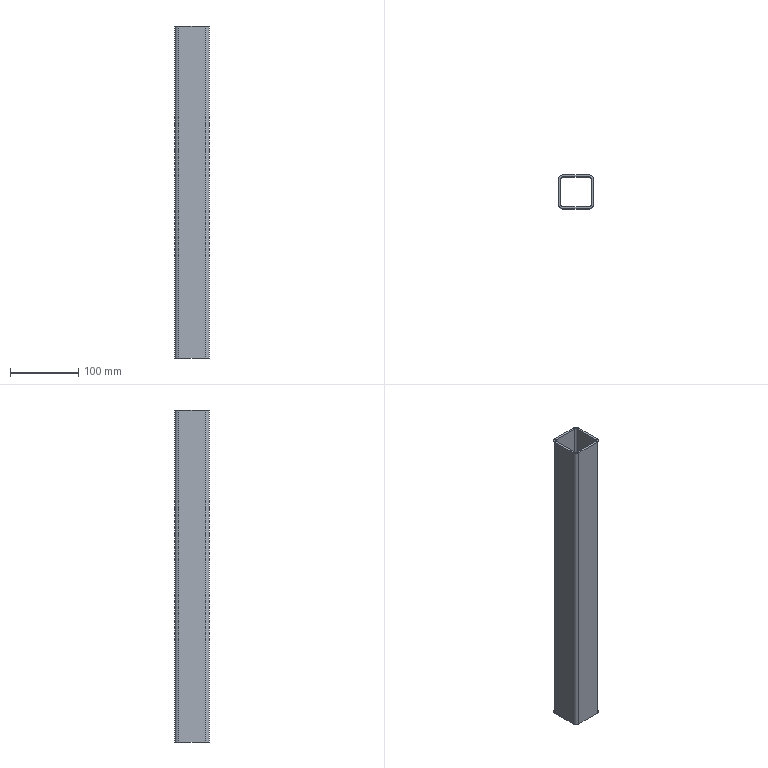Part | SolidWorks | 1 solid | 18 faces | box 50 x 50 x 485 mm | volume 262299 mm3 | plane 10 | cylinder 8 | commonest cylinder face diameters 6 x4 12 x4
STEP:
#1=CARTESIAN_POINT('',(19.,25.,242.5));
#2=VERTEX_POINT('',#1);
#3=CARTESIAN_POINT('',(25.,19.,242.5));
#4=VERTEX_POINT('',#3);
#5=CARTESIAN_POINT('',(19.,19.,242.5));
#6=DIRECTION('',(0.,0.,-1.));
#7=DIRECTION('',(-1.,0.,0.));
#8=AXIS2_PLACEMENT_3D('',#5,#6,#7);
#9=CIRCLE('',#8,6.);
#10=EDGE_CURVE('',#2,#4,#9,.T.);
#11=ORIENTED_EDGE('',*,*,#10,.T.);
#12=CARTESIAN_POINT('',(25.,19.,-242.5));
#13=VERTEX_POINT('',#12);
#14=CARTESIAN_POINT('',(25.,19.,-242.5));
#15=DIRECTION('',(0.,0.,1.));
#16=VECTOR('',#15,1000.);
#17=LINE('',#14,#16);
#18=EDGE_CURVE('',#13,#4,#17,.T.);
#19=ORIENTED_EDGE('',*,*,#18,.F.);
#20=CARTESIAN_POINT('',(19.,25.,-242.5));
#21=VERTEX_POINT('',#20);
#22=CARTESIAN_POINT('',(19.,19.,-242.5));
#23=DIRECTION('',(0.,0.,-1.));
#24=DIRECTION('',(-1.,0.,0.));
#25=AXIS2_PLACEMENT_3D('',#22,#23,#24);
#26=CIRCLE('',#25,6.);
#27=EDGE_CURVE('',#21,#13,#26,.T.);
#28=ORIENTED_EDGE('',*,*,#27,.F.);
#29=CARTESIAN_POINT('',(19.,25.,-242.5));
#30=DIRECTION('',(0.,0.,1.));
#31=VECTOR('',#30,1000.);
#32=LINE('',#29,#31);
#33=EDGE_CURVE('',#21,#2,#32,.T.);
#34=ORIENTED_EDGE('',*,*,#33,.T.);
#35=EDGE_LOOP('',(#11,#19,#28,#34));
#36=FACE_OUTER_BOUND('',#35,.T.);
#37=CARTESIAN_POINT('',(19.,19.,-242.5));
#38=DIRECTION('',(0.,0.,1.));
#39=DIRECTION('',(1.,0.,0.));
#40=AXIS2_PLACEMENT_3D('',#37,#38,#39);
#41=CYLINDRICAL_SURFACE('',#40,6.);
#42=ADVANCED_FACE('',(#36),#41,.T.);
#43=CARTESIAN_POINT('',(25.,-19.,242.5));
#44=VERTEX_POINT('',#43);
#45=CARTESIAN_POINT('',(25.,19.,242.5));
#46=DIRECTION('',(0.,-1.,0.));
#47=VECTOR('',#46,1000.);
#48=LINE('',#45,#47);
#49=EDGE_CURVE('',#4,#44,#48,.T.);
#50=ORIENTED_EDGE('',*,*,#49,.T.);
#51=CARTESIAN_POINT('',(25.,-19.,-242.5));
#52=VERTEX_POINT('',#51);
#53=CARTESIAN_POINT('',(25.,-19.,-242.5));
#54=DIRECTION('',(0.,0.,1.));
#55=VECTOR('',#54,1000.);
#56=LINE('',#53,#55);
#57=EDGE_CURVE('',#52,#44,#56,.T.);
#58=ORIENTED_EDGE('',*,*,#57,.F.);
#59=CARTESIAN_POINT('',(25.,19.,-242.5));
#60=DIRECTION('',(0.,-1.,0.));
#61=VECTOR('',#60,1000.);
#62=LINE('',#59,#61);
#63=EDGE_CURVE('',#13,#52,#62,.T.);
#64=ORIENTED_EDGE('',*,*,#63,.F.);
#65=ORIENTED_EDGE('',*,*,#18,.T.);
#66=EDGE_LOOP('',(#50,#58,#64,#65));
#67=FACE_OUTER_BOUND('',#66,.T.);
#68=CARTESIAN_POINT('',(25.,19.,-242.5));
#69=DIRECTION('',(-1.,0.,0.));
#70=DIRECTION('',(0.,0.,1.));
#71=AXIS2_PLACEMENT_3D('',#68,#69,#70);
#72=PLANE('',#71);
#73=ADVANCED_FACE('',(#67),#72,.F.);
#74=CARTESIAN_POINT('',(19.,-25.,242.5));
#75=VERTEX_POINT('',#74);
#76=CARTESIAN_POINT('',(19.,-19.,242.5));
#77=DIRECTION('',(0.,0.,-1.));
#78=DIRECTION('',(-1.,0.,0.));
#79=AXIS2_PLACEMENT_3D('',#76,#77,#78);
#80=CIRCLE('',#79,6.);
#81=EDGE_CURVE('',#44,#75,#80,.T.);
#82=ORIENTED_EDGE('',*,*,#81,.T.);
#83=CARTESIAN_POINT('',(19.,-25.,-242.5));
#84=VERTEX_POINT('',#83);
#85=CARTESIAN_POINT('',(19.,-25.,-242.5));
#86=DIRECTION('',(0.,0.,1.));
#87=VECTOR('',#86,1000.);
#88=LINE('',#85,#87);
#89=EDGE_CURVE('',#84,#75,#88,.T.);
#90=ORIENTED_EDGE('',*,*,#89,.F.);
#91=CARTESIAN_POINT('',(19.,-19.,-242.5));
#92=DIRECTION('',(0.,0.,-1.));
#93=DIRECTION('',(-1.,0.,0.));
#94=AXIS2_PLACEMENT_3D('',#91,#92,#93);
#95=CIRCLE('',#94,6.);
#96=EDGE_CURVE('',#52,#84,#95,.T.);
#97=ORIENTED_EDGE('',*,*,#96,.F.);
#98=ORIENTED_EDGE('',*,*,#57,.T.);
#99=EDGE_LOOP('',(#82,#90,#97,#98));
#100=FACE_OUTER_BOUND('',#99,.T.);
#101=CARTESIAN_POINT('',(19.,-19.,-242.5));
#102=DIRECTION('',(0.,0.,1.));
#103=DIRECTION('',(1.,0.,0.));
#104=AXIS2_PLACEMENT_3D('',#101,#102,#103);
#105=CYLINDRICAL_SURFACE('',#104,6.);
#106=ADVANCED_FACE('',(#100),#105,.T.);
#107=CARTESIAN_POINT('',(-19.,-25.,242.5));
#108=VERTEX_POINT('',#107);
#109=CARTESIAN_POINT('',(-19.,-25.,242.5));
#110=DIRECTION('',(-1.,0.,0.));
#111=VECTOR('',#110,1000.);
#112=LINE('',#109,#111);
#113=EDGE_CURVE('',#75,#108,#112,.T.);
#114=ORIENTED_EDGE('',*,*,#113,.T.);
#115=CARTESIAN_POINT('',(-19.,-25.,-242.5));
#116=VERTEX_POINT('',#115);
#117=CARTESIAN_POINT('',(-19.,-25.,-242.5));
#118=DIRECTION('',(0.,0.,1.));
#119=VECTOR('',#118,1000.);
#120=LINE('',#117,#119);
#121=EDGE_CURVE('',#116,#108,#120,.T.);
#122=ORIENTED_EDGE('',*,*,#121,.F.);
#123=CARTESIAN_POINT('',(-19.,-25.,-242.5));
#124=DIRECTION('',(-1.,0.,0.));
#125=VECTOR('',#124,1000.);
#126=LINE('',#123,#125);
#127=EDGE_CURVE('',#84,#116,#126,.T.);
#128=ORIENTED_EDGE('',*,*,#127,.F.);
#129=ORIENTED_EDGE('',*,*,#89,.T.);
#130=EDGE_LOOP('',(#114,#122,#128,#129));
#131=FACE_OUTER_BOUND('',#130,.T.);
#132=CARTESIAN_POINT('',(-19.,-25.,-242.5));
#133=DIRECTION('',(0.,1.,0.));
#134=DIRECTION('',(0.,0.,1.));
#135=AXIS2_PLACEMENT_3D('',#132,#133,#134);
#136=PLANE('',#135);
#137=ADVANCED_FACE('',(#131),#136,.F.);
#138=CARTESIAN_POINT('',(-25.,-19.,242.5));
#139=VERTEX_POINT('',#138);
#140=CARTESIAN_POINT('',(-19.,-19.,242.5));
#141=DIRECTION('',(0.,0.,-1.));
#142=DIRECTION('',(-1.,0.,0.));
#143=AXIS2_PLACEMENT_3D('',#140,#141,#142);
#144=CIRCLE('',#143,6.);
#145=EDGE_CURVE('',#108,#139,#144,.T.);
#146=ORIENTED_EDGE('',*,*,#145,.T.);
#147=CARTESIAN_POINT('',(-25.,-19.,-242.5));
#148=VERTEX_POINT('',#147);
#149=CARTESIAN_POINT('',(-25.,-19.,-242.5));
#150=DIRECTION('',(0.,0.,1.));
#151=VECTOR('',#150,1000.);
#152=LINE('',#149,#151);
#153=EDGE_CURVE('',#148,#139,#152,.T.);
#154=ORIENTED_EDGE('',*,*,#153,.F.);
#155=CARTESIAN_POINT('',(-19.,-19.,-242.5));
#156=DIRECTION('',(0.,0.,-1.));
#157=DIRECTION('',(-1.,0.,0.));
#158=AXIS2_PLACEMENT_3D('',#155,#156,#157);
#159=CIRCLE('',#158,6.);
#160=EDGE_CURVE('',#116,#148,#159,.T.);
#161=ORIENTED_EDGE('',*,*,#160,.F.);
#162=ORIENTED_EDGE('',*,*,#121,.T.);
#163=EDGE_LOOP('',(#146,#154,#161,#162));
#164=FACE_OUTER_BOUND('',#163,.T.);
#165=CARTESIAN_POINT('',(-19.,-19.,-242.5));
#166=DIRECTION('',(0.,0.,1.));
#167=DIRECTION('',(1.,0.,0.));
#168=AXIS2_PLACEMENT_3D('',#165,#166,#167);
#169=CYLINDRICAL_SURFACE('',#168,6.);
#170=ADVANCED_FACE('',(#164),#169,.T.);
#171=CARTESIAN_POINT('',(-25.,19.,242.5));
#172=VERTEX_POINT('',#171);
#173=CARTESIAN_POINT('',(-25.,-19.,242.5));
#174=DIRECTION('',(0.,1.,0.));
#175=VECTOR('',#174,1000.);
#176=LINE('',#173,#175);
#177=EDGE_CURVE('',#139,#172,#176,.T.);
#178=ORIENTED_EDGE('',*,*,#177,.T.);
#179=CARTESIAN_POINT('',(-25.,19.,-242.5));
#180=VERTEX_POINT('',#179);
#181=CARTESIAN_POINT('',(-25.,19.,-242.5));
#182=DIRECTION('',(0.,0.,1.));
#183=VECTOR('',#182,1000.);
#184=LINE('',#181,#183);
#185=EDGE_CURVE('',#180,#172,#184,.T.);
#186=ORIENTED_EDGE('',*,*,#185,.F.);
#187=CARTESIAN_POINT('',(-25.,-19.,-242.5));
#188=DIRECTION('',(0.,1.,0.));
#189=VECTOR('',#188,1000.);
#190=LINE('',#187,#189);
#191=EDGE_CURVE('',#148,#180,#190,.T.);
#192=ORIENTED_EDGE('',*,*,#191,.F.);
#193=ORIENTED_EDGE('',*,*,#153,.T.);
#194=EDGE_LOOP('',(#178,#186,#192,#193));
#195=FACE_OUTER_BOUND('',#194,.T.);
#196=CARTESIAN_POINT('',(-25.,-19.,-242.5));
#197=DIRECTION('',(1.,0.,0.));
#198=DIRECTION('',(0.,0.,-1.));
#199=AXIS2_PLACEMENT_3D('',#196,#197,#198);
#200=PLANE('',#199);
#201=ADVANCED_FACE('',(#195),#200,.F.);
#202=CARTESIAN_POINT('',(-19.,25.,242.5));
#203=VERTEX_POINT('',#202);
#204=CARTESIAN_POINT('',(-19.,19.,242.5));
#205=DIRECTION('',(0.,0.,-1.));
#206=DIRECTION('',(-1.,0.,0.));
#207=AXIS2_PLACEMENT_3D('',#204,#205,#206);
#208=CIRCLE('',#207,6.);
#209=EDGE_CURVE('',#172,#203,#208,.T.);
#210=ORIENTED_EDGE('',*,*,#209,.T.);
#211=CARTESIAN_POINT('',(-19.,25.,-242.5));
#212=VERTEX_POINT('',#211);
#213=CARTESIAN_POINT('',(-19.,25.,-242.5));
#214=DIRECTION('',(0.,0.,1.));
#215=VECTOR('',#214,1000.);
#216=LINE('',#213,#215);
#217=EDGE_CURVE('',#212,#203,#216,.T.);
#218=ORIENTED_EDGE('',*,*,#217,.F.);
#219=CARTESIAN_POINT('',(-19.,19.,-242.5));
#220=DIRECTION('',(0.,0.,-1.));
#221=DIRECTION('',(-1.,0.,0.));
#222=AXIS2_PLACEMENT_3D('',#219,#220,#221);
#223=CIRCLE('',#222,6.);
#224=EDGE_CURVE('',#180,#212,#223,.T.);
#225=ORIENTED_EDGE('',*,*,#224,.F.);
#226=ORIENTED_EDGE('',*,*,#185,.T.);
#227=EDGE_LOOP('',(#210,#218,#225,#226));
#228=FACE_OUTER_BOUND('',#227,.T.);
#229=CARTESIAN_POINT('',(-19.,19.,-242.5));
#230=DIRECTION('',(0.,0.,1.));
#231=DIRECTION('',(1.,0.,0.));
#232=AXIS2_PLACEMENT_3D('',#229,#230,#231);
#233=CYLINDRICAL_SURFACE('',#232,6.);
#234=ADVANCED_FACE('',(#228),#233,.T.);
#235=CARTESIAN_POINT('',(22.,-19.,242.5));
#236=VERTEX_POINT('',#235);
#237=CARTESIAN_POINT('',(19.,-22.,242.5));
#238=VERTEX_POINT('',#237);
#239=CARTESIAN_POINT('',(19.,-19.,242.5));
#240=DIRECTION('',(0.,0.,-1.));
#241=DIRECTION('',(-1.,0.,0.));
#242=AXIS2_PLACEMENT_3D('',#239,#240,#241);
#243=CIRCLE('',#242,3.);
#244=EDGE_CURVE('',#236,#238,#243,.T.);
#245=ORIENTED_EDGE('',*,*,#244,.F.);
#246=CARTESIAN_POINT('',(22.,-19.,-242.5));
#247=VERTEX_POINT('',#246);
#248=CARTESIAN_POINT('',(22.,-19.,-242.5));
#249=DIRECTION('',(0.,0.,1.));
#250=VECTOR('',#249,1000.);
#251=LINE('',#248,#250);
#252=EDGE_CURVE('',#247,#236,#251,.T.);
#253=ORIENTED_EDGE('',*,*,#252,.F.);
#254=CARTESIAN_POINT('',(19.,-22.,-242.5));
#255=VERTEX_POINT('',#254);
#256=CARTESIAN_POINT('',(19.,-19.,-242.5));
#257=DIRECTION('',(0.,0.,-1.));
#258=DIRECTION('',(-1.,0.,0.));
#259=AXIS2_PLACEMENT_3D('',#256,#257,#258);
#260=CIRCLE('',#259,3.);
#261=EDGE_CURVE('',#247,#255,#260,.T.);
#262=ORIENTED_EDGE('',*,*,#261,.T.);
#263=CARTESIAN_POINT('',(19.,-22.,-242.5));
#264=DIRECTION('',(0.,0.,1.));
#265=VECTOR('',#264,1000.);
#266=LINE('',#263,#265);
#267=EDGE_CURVE('',#255,#238,#266,.T.);
#268=ORIENTED_EDGE('',*,*,#267,.T.);
#269=EDGE_LOOP('',(#245,#253,#262,#268));
#270=FACE_OUTER_BOUND('',#269,.T.);
#271=CARTESIAN_POINT('',(19.,-19.,-242.5));
#272=DIRECTION('',(0.,0.,1.));
#273=DIRECTION('',(1.,0.,0.));
#274=AXIS2_PLACEMENT_3D('',#271,#272,#273);
#275=CYLINDRICAL_SURFACE('',#274,3.);
#276=ADVANCED_FACE('',(#270),#275,.F.);
#277=CARTESIAN_POINT('',(22.,19.,242.5));
#278=VERTEX_POINT('',#277);
#279=CARTESIAN_POINT('',(22.,19.,242.5));
#280=DIRECTION('',(0.,-1.,0.));
#281=VECTOR('',#280,1000.);
#282=LINE('',#279,#281);
#283=EDGE_CURVE('',#278,#236,#282,.T.);
#284=ORIENTED_EDGE('',*,*,#283,.F.);
#285=CARTESIAN_POINT('',(22.,19.,-242.5));
#286=VERTEX_POINT('',#285);
#287=CARTESIAN_POINT('',(22.,19.,-242.5));
#288=DIRECTION('',(0.,0.,1.));
#289=VECTOR('',#288,1000.);
#290=LINE('',#287,#289);
#291=EDGE_CURVE('',#286,#278,#290,.T.);
#292=ORIENTED_EDGE('',*,*,#291,.F.);
#293=CARTESIAN_POINT('',(22.,19.,-242.5));
#294=DIRECTION('',(0.,-1.,0.));
#295=VECTOR('',#294,1000.);
#296=LINE('',#293,#295);
#297=EDGE_CURVE('',#286,#247,#296,.T.);
#298=ORIENTED_EDGE('',*,*,#297,.T.);
#299=ORIENTED_EDGE('',*,*,#252,.T.);
#300=EDGE_LOOP('',(#284,#292,#298,#299));
#301=FACE_OUTER_BOUND('',#300,.T.);
#302=CARTESIAN_POINT('',(22.,19.,-242.5));
#303=DIRECTION('',(-1.,0.,0.));
#304=DIRECTION('',(0.,0.,1.));
#305=AXIS2_PLACEMENT_3D('',#302,#303,#304);
#306=PLANE('',#305);
#307=ADVANCED_FACE('',(#301),#306,.T.);
#308=CARTESIAN_POINT('',(19.,22.,242.5));
#309=VERTEX_POINT('',#308);
#310=CARTESIAN_POINT('',(19.,19.,242.5));
#311=DIRECTION('',(0.,0.,-1.));
#312=DIRECTION('',(-1.,0.,0.));
#313=AXIS2_PLACEMENT_3D('',#310,#311,#312);
#314=CIRCLE('',#313,3.);
#315=EDGE_CURVE('',#309,#278,#314,.T.);
#316=ORIENTED_EDGE('',*,*,#315,.F.);
#317=CARTESIAN_POINT('',(19.,22.,-242.5));
#318=VERTEX_POINT('',#317);
#319=CARTESIAN_POINT('',(19.,22.,-242.5));
#320=DIRECTION('',(0.,0.,1.));
#321=VECTOR('',#320,1000.);
#322=LINE('',#319,#321);
#323=EDGE_CURVE('',#318,#309,#322,.T.);
#324=ORIENTED_EDGE('',*,*,#323,.F.);
#325=CARTESIAN_POINT('',(19.,19.,-242.5));
#326=DIRECTION('',(0.,0.,-1.));
#327=DIRECTION('',(-1.,0.,0.));
#328=AXIS2_PLACEMENT_3D('',#325,#326,#327);
#329=CIRCLE('',#328,3.);
#330=EDGE_CURVE('',#318,#286,#329,.T.);
#331=ORIENTED_EDGE('',*,*,#330,.T.);
#332=ORIENTED_EDGE('',*,*,#291,.T.);
#333=EDGE_LOOP('',(#316,#324,#331,#332));
#334=FACE_OUTER_BOUND('',#333,.T.);
#335=CARTESIAN_POINT('',(19.,19.,-242.5));
#336=DIRECTION('',(0.,0.,1.));
#337=DIRECTION('',(1.,0.,0.));
#338=AXIS2_PLACEMENT_3D('',#335,#336,#337);
#339=CYLINDRICAL_SURFACE('',#338,3.);
#340=ADVANCED_FACE('',(#334),#339,.F.);
#341=CARTESIAN_POINT('',(-19.,22.,242.5));
#342=VERTEX_POINT('',#341);
#343=CARTESIAN_POINT('',(19.,22.,242.5));
#344=DIRECTION('',(1.,0.,0.));
#345=VECTOR('',#344,1000.);
#346=LINE('',#343,#345);
#347=EDGE_CURVE('',#342,#309,#346,.T.);
#348=ORIENTED_EDGE('',*,*,#347,.F.);
#349=CARTESIAN_POINT('',(-19.,22.,-242.5));
#350=VERTEX_POINT('',#349);
#351=CARTESIAN_POINT('',(-19.,22.,-242.5));
#352=DIRECTION('',(0.,0.,1.));
#353=VECTOR('',#352,1000.);
#354=LINE('',#351,#353);
#355=EDGE_CURVE('',#350,#342,#354,.T.);
#356=ORIENTED_EDGE('',*,*,#355,.F.);
#357=CARTESIAN_POINT('',(19.,22.,-242.5));
#358=DIRECTION('',(1.,0.,0.));
#359=VECTOR('',#358,1000.);
#360=LINE('',#357,#359);
#361=EDGE_CURVE('',#350,#318,#360,.T.);
#362=ORIENTED_EDGE('',*,*,#361,.T.);
#363=ORIENTED_EDGE('',*,*,#323,.T.);
#364=EDGE_LOOP('',(#348,#356,#362,#363));
#365=FACE_OUTER_BOUND('',#364,.T.);
#366=CARTESIAN_POINT('',(19.,22.,-242.5));
#367=DIRECTION('',(0.,-1.,0.));
#368=DIRECTION('',(0.,0.,-1.));
#369=AXIS2_PLACEMENT_3D('',#366,#367,#368);
#370=PLANE('',#369);
#371=ADVANCED_FACE('',(#365),#370,.T.);
#372=CARTESIAN_POINT('',(-22.,19.,242.5));
#373=VERTEX_POINT('',#372);
#374=CARTESIAN_POINT('',(-19.,19.,242.5));
#375=DIRECTION('',(0.,0.,-1.));
#376=DIRECTION('',(-1.,0.,0.));
#377=AXIS2_PLACEMENT_3D('',#374,#375,#376);
#378=CIRCLE('',#377,3.);
#379=EDGE_CURVE('',#373,#342,#378,.T.);
#380=ORIENTED_EDGE('',*,*,#379,.F.);
#381=CARTESIAN_POINT('',(-22.,19.,-242.5));
#382=VERTEX_POINT('',#381);
#383=CARTESIAN_POINT('',(-22.,19.,-242.5));
#384=DIRECTION('',(0.,0.,1.));
#385=VECTOR('',#384,1000.);
#386=LINE('',#383,#385);
#387=EDGE_CURVE('',#382,#373,#386,.T.);
#388=ORIENTED_EDGE('',*,*,#387,.F.);
#389=CARTESIAN_POINT('',(-19.,19.,-242.5));
#390=DIRECTION('',(0.,0.,-1.));
#391=DIRECTION('',(-1.,0.,0.));
#392=AXIS2_PLACEMENT_3D('',#389,#390,#391);
#393=CIRCLE('',#392,3.);
#394=EDGE_CURVE('',#382,#350,#393,.T.);
#395=ORIENTED_EDGE('',*,*,#394,.T.);
#396=ORIENTED_EDGE('',*,*,#355,.T.);
#397=EDGE_LOOP('',(#380,#388,#395,#396));
#398=FACE_OUTER_BOUND('',#397,.T.);
#399=CARTESIAN_POINT('',(-19.,19.,-242.5));
#400=DIRECTION('',(0.,0.,1.));
#401=DIRECTION('',(1.,0.,0.));
#402=AXIS2_PLACEMENT_3D('',#399,#400,#401);
#403=CYLINDRICAL_SURFACE('',#402,3.);
#404=ADVANCED_FACE('',(#398),#403,.F.);
#405=CARTESIAN_POINT('',(-22.,-19.,242.5));
#406=VERTEX_POINT('',#405);
#407=CARTESIAN_POINT('',(-22.,-19.,242.5));
#408=DIRECTION('',(0.,1.,0.));
#409=VECTOR('',#408,1000.);
#410=LINE('',#407,#409);
#411=EDGE_CURVE('',#406,#373,#410,.T.);
#412=ORIENTED_EDGE('',*,*,#411,.F.);
#413=CARTESIAN_POINT('',(-22.,-19.,-242.5));
#414=VERTEX_POINT('',#413);
#415=CARTESIAN_POINT('',(-22.,-19.,-242.5));
#416=DIRECTION('',(0.,0.,1.));
#417=VECTOR('',#416,1000.);
#418=LINE('',#415,#417);
#419=EDGE_CURVE('',#414,#406,#418,.T.);
#420=ORIENTED_EDGE('',*,*,#419,.F.);
#421=CARTESIAN_POINT('',(-22.,-19.,-242.5));
#422=DIRECTION('',(0.,1.,0.));
#423=VECTOR('',#422,1000.);
#424=LINE('',#421,#423);
#425=EDGE_CURVE('',#414,#382,#424,.T.);
#426=ORIENTED_EDGE('',*,*,#425,.T.);
#427=ORIENTED_EDGE('',*,*,#387,.T.);
#428=EDGE_LOOP('',(#412,#420,#426,#427));
#429=FACE_OUTER_BOUND('',#428,.T.);
#430=CARTESIAN_POINT('',(-22.,-19.,-242.5));
#431=DIRECTION('',(1.,0.,0.));
#432=DIRECTION('',(0.,0.,-1.));
#433=AXIS2_PLACEMENT_3D('',#430,#431,#432);
#434=PLANE('',#433);
#435=ADVANCED_FACE('',(#429),#434,.T.);
#436=CARTESIAN_POINT('',(-19.,-22.,242.5));
#437=VERTEX_POINT('',#436);
#438=CARTESIAN_POINT('',(-19.,-19.,242.5));
#439=DIRECTION('',(0.,0.,-1.));
#440=DIRECTION('',(-1.,0.,0.));
#441=AXIS2_PLACEMENT_3D('',#438,#439,#440);
#442=CIRCLE('',#441,3.);
#443=EDGE_CURVE('',#437,#406,#442,.T.);
#444=ORIENTED_EDGE('',*,*,#443,.F.);
#445=CARTESIAN_POINT('',(-19.,-22.,-242.5));
#446=VERTEX_POINT('',#445);
#447=CARTESIAN_POINT('',(-19.,-22.,-242.5));
#448=DIRECTION('',(0.,0.,1.));
#449=VECTOR('',#448,1000.);
#450=LINE('',#447,#449);
#451=EDGE_CURVE('',#446,#437,#450,.T.);
#452=ORIENTED_EDGE('',*,*,#451,.F.);
#453=CARTESIAN_POINT('',(-19.,-19.,-242.5));
#454=DIRECTION('',(0.,0.,-1.));
#455=DIRECTION('',(-1.,0.,0.));
#456=AXIS2_PLACEMENT_3D('',#453,#454,#455);
#457=CIRCLE('',#456,3.);
#458=EDGE_CURVE('',#446,#414,#457,.T.);
#459=ORIENTED_EDGE('',*,*,#458,.T.);
#460=ORIENTED_EDGE('',*,*,#419,.T.);
#461=EDGE_LOOP('',(#444,#452,#459,#460));
#462=FACE_OUTER_BOUND('',#461,.T.);
#463=CARTESIAN_POINT('',(-19.,-19.,-242.5));
#464=DIRECTION('',(0.,0.,1.));
#465=DIRECTION('',(1.,0.,0.));
#466=AXIS2_PLACEMENT_3D('',#463,#464,#465);
#467=CYLINDRICAL_SURFACE('',#466,3.);
#468=ADVANCED_FACE('',(#462),#467,.F.);
#469=CARTESIAN_POINT('',(-19.,-22.,242.5));
#470=DIRECTION('',(-1.,0.,0.));
#471=VECTOR('',#470,1000.);
#472=LINE('',#469,#471);
#473=EDGE_CURVE('',#238,#437,#472,.T.);
#474=ORIENTED_EDGE('',*,*,#473,.F.);
#475=ORIENTED_EDGE('',*,*,#267,.F.);
#476=CARTESIAN_POINT('',(-19.,-22.,-242.5));
#477=DIRECTION('',(-1.,0.,0.));
#478=VECTOR('',#477,1000.);
#479=LINE('',#476,#478);
#480=EDGE_CURVE('',#255,#446,#479,.T.);
#481=ORIENTED_EDGE('',*,*,#480,.T.);
#482=ORIENTED_EDGE('',*,*,#451,.T.);
#483=EDGE_LOOP('',(#474,#475,#481,#482));
#484=FACE_OUTER_BOUND('',#483,.T.);
#485=CARTESIAN_POINT('',(-19.,-22.,-242.5));
#486=DIRECTION('',(0.,1.,0.));
#487=DIRECTION('',(0.,0.,1.));
#488=AXIS2_PLACEMENT_3D('',#485,#486,#487);
#489=PLANE('',#488);
#490=ADVANCED_FACE('',(#484),#489,.T.);
#491=CARTESIAN_POINT('',(19.,25.,242.5));
#492=DIRECTION('',(1.,0.,0.));
#493=VECTOR('',#492,1000.);
#494=LINE('',#491,#493);
#495=EDGE_CURVE('',#203,#2,#494,.T.);
#496=ORIENTED_EDGE('',*,*,#495,.T.);
#497=ORIENTED_EDGE('',*,*,#33,.F.);
#498=CARTESIAN_POINT('',(19.,25.,-242.5));
#499=DIRECTION('',(1.,0.,0.));
#500=VECTOR('',#499,1000.);
#501=LINE('',#498,#500);
#502=EDGE_CURVE('',#212,#21,#501,.T.);
#503=ORIENTED_EDGE('',*,*,#502,.F.);
#504=ORIENTED_EDGE('',*,*,#217,.T.);
#505=EDGE_LOOP('',(#496,#497,#503,#504));
#506=FACE_OUTER_BOUND('',#505,.T.);
#507=CARTESIAN_POINT('',(19.,25.,-242.5));
#508=DIRECTION('',(0.,-1.,0.));
#509=DIRECTION('',(0.,0.,-1.));
#510=AXIS2_PLACEMENT_3D('',#507,#508,#509);
#511=PLANE('',#510);
#512=ADVANCED_FACE('',(#506),#511,.F.);
#513=ORIENTED_EDGE('',*,*,#261,.F.);
#514=ORIENTED_EDGE('',*,*,#297,.F.);
#515=ORIENTED_EDGE('',*,*,#330,.F.);
#516=ORIENTED_EDGE('',*,*,#361,.F.);
#517=ORIENTED_EDGE('',*,*,#394,.F.);
#518=ORIENTED_EDGE('',*,*,#425,.F.);
#519=ORIENTED_EDGE('',*,*,#458,.F.);
#520=ORIENTED_EDGE('',*,*,#480,.F.);
#521=EDGE_LOOP('',(#513,#514,#515,#516,#517,#518,#519,#520));
#522=FACE_BOUND('',#521,.T.);
#523=ORIENTED_EDGE('',*,*,#27,.T.);
#524=ORIENTED_EDGE('',*,*,#63,.T.);
#525=ORIENTED_EDGE('',*,*,#96,.T.);
#526=ORIENTED_EDGE('',*,*,#127,.T.);
#527=ORIENTED_EDGE('',*,*,#160,.T.);
#528=ORIENTED_EDGE('',*,*,#191,.T.);
#529=ORIENTED_EDGE('',*,*,#224,.T.);
#530=ORIENTED_EDGE('',*,*,#502,.T.);
#531=EDGE_LOOP('',(#523,#524,#525,#526,#527,#528,#529,#530));
#532=FACE_OUTER_BOUND('',#531,.T.);
#533=CARTESIAN_POINT('',(19.,19.,-242.5));
#534=DIRECTION('',(0.,0.,-1.));
#535=DIRECTION('',(-1.,0.,0.));
#536=AXIS2_PLACEMENT_3D('',#533,#534,#535);
#537=PLANE('',#536);
#538=ADVANCED_FACE('',(#522,#532),#537,.T.);
#539=ORIENTED_EDGE('',*,*,#244,.T.);
#540=ORIENTED_EDGE('',*,*,#473,.T.);
#541=ORIENTED_EDGE('',*,*,#443,.T.);
#542=ORIENTED_EDGE('',*,*,#411,.T.);
#543=ORIENTED_EDGE('',*,*,#379,.T.);
#544=ORIENTED_EDGE('',*,*,#347,.T.);
#545=ORIENTED_EDGE('',*,*,#315,.T.);
#546=ORIENTED_EDGE('',*,*,#283,.T.);
#547=EDGE_LOOP('',(#539,#540,#541,#542,#543,#544,#545,#546));
#548=FACE_BOUND('',#547,.T.);
#549=ORIENTED_EDGE('',*,*,#10,.F.);
#550=ORIENTED_EDGE('',*,*,#495,.F.);
#551=ORIENTED_EDGE('',*,*,#209,.F.);
#552=ORIENTED_EDGE('',*,*,#177,.F.);
#553=ORIENTED_EDGE('',*,*,#145,.F.);
#554=ORIENTED_EDGE('',*,*,#113,.F.);
#555=ORIENTED_EDGE('',*,*,#81,.F.);
#556=ORIENTED_EDGE('',*,*,#49,.F.);
#557=EDGE_LOOP('',(#549,#550,#551,#552,#553,#554,#555,#556));
#558=FACE_OUTER_BOUND('',#557,.T.);
#559=CARTESIAN_POINT('',(19.,19.,242.5));
#560=DIRECTION('',(0.,0.,-1.));
#561=DIRECTION('',(-1.,0.,0.));
#562=AXIS2_PLACEMENT_3D('',#559,#560,#561);
#563=PLANE('',#562);
#564=ADVANCED_FACE('',(#548,#558),#563,.F.);
#565=CLOSED_SHELL('',(#42,#73,#106,#137,#170,#201,#234,#276,#307,#340,#371,#404,#435,#468,#490,#512,#538,#564));
#566=MANIFOLD_SOLID_BREP('',#565);
#567=CARTESIAN_POINT('',(0.,0.,0.));
#568=DIRECTION('',(0.,0.,1.));
#569=DIRECTION('',(1.,0.,0.));
#570=AXIS2_PLACEMENT_3D('',#567,#568,#569);
#571=(LENGTH_UNIT()NAMED_UNIT(*)SI_UNIT(.MILLI.,.METRE.));
#572=UNCERTAINTY_MEASURE_WITH_UNIT(LENGTH_MEASURE(0.00001),#571,'','');
#573=(NAMED_UNIT(*)PLANE_ANGLE_UNIT()SI_UNIT($,.RADIAN.));
#574=(NAMED_UNIT(*)SI_UNIT($,.STERADIAN.)SOLID_ANGLE_UNIT());
#575=(GEOMETRIC_REPRESENTATION_CONTEXT(3)GLOBAL_UNCERTAINTY_ASSIGNED_CONTEXT((#572))GLOBAL_UNIT_ASSIGNED_CONTEXT((#571,#573,#574))REPRESENTATION_CONTEXT('',''));
#576=ADVANCED_BREP_SHAPE_REPRESENTATION('',(#566,#570),#575);